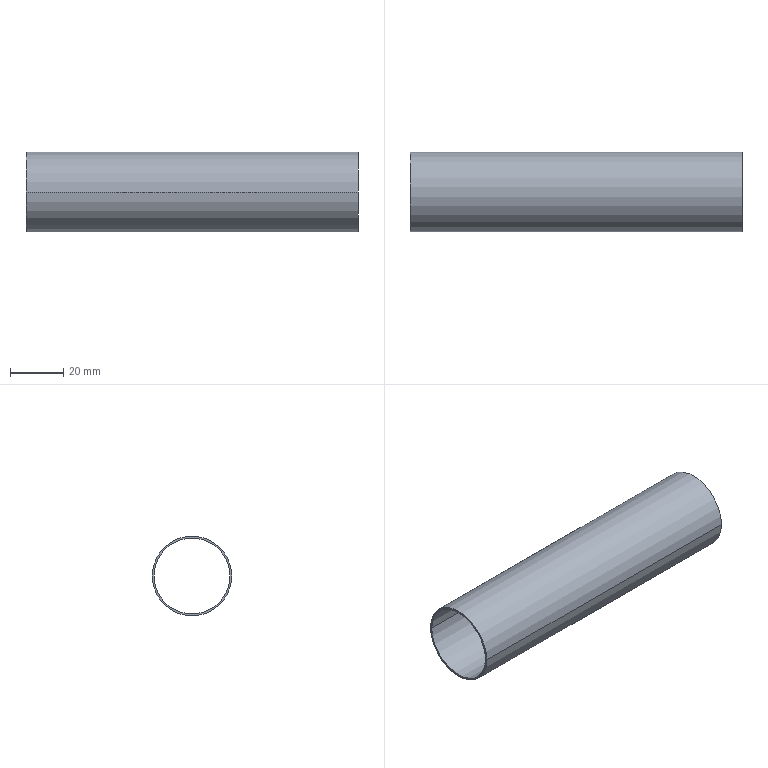Part | STEP file | Component4_2 | 1 solid | 6 faces | box 125 x 30 x 30 mm | volume 8054 mm3 | cylinder 4 | plane 2 | commonest cylinder face diameters 28.6 x2 30 x2
STEP:
#1=CARTESIAN_POINT('',(140.,140.7,17.));
#2=VERTEX_POINT('',#1);
#3=CARTESIAN_POINT('',(140.,169.3,17.));
#4=VERTEX_POINT('',#3);
#5=CARTESIAN_POINT('',(140.,155.,17.));
#6=DIRECTION('',(-1.,0.,0.));
#7=DIRECTION('',(0.,1.,0.));
#8=AXIS2_PLACEMENT_3D('',#5,#6,#7);
#9=CIRCLE('',#8,14.3);
#10=EDGE_CURVE('',#2,#4,#9,.T.);
#11=ORIENTED_EDGE('',*,*,#10,.F.);
#12=CARTESIAN_POINT('',(15.,140.7,17.));
#13=VERTEX_POINT('',#12);
#14=CARTESIAN_POINT('',(140.,140.7,17.));
#15=DIRECTION('',(-1.,0.,0.));
#16=VECTOR('',#15,1000.);
#17=LINE('',#14,#16);
#18=EDGE_CURVE('',#2,#13,#17,.T.);
#19=ORIENTED_EDGE('',*,*,#18,.T.);
#20=CARTESIAN_POINT('',(15.,169.3,17.));
#21=VERTEX_POINT('',#20);
#22=CARTESIAN_POINT('',(15.,155.,17.));
#23=DIRECTION('',(1.,0.,0.));
#24=DIRECTION('',(0.,1.,0.));
#25=AXIS2_PLACEMENT_3D('',#22,#23,#24);
#26=CIRCLE('',#25,14.3);
#27=EDGE_CURVE('',#21,#13,#26,.T.);
#28=ORIENTED_EDGE('',*,*,#27,.F.);
#29=CARTESIAN_POINT('',(140.,169.3,17.));
#30=DIRECTION('',(-1.,0.,0.));
#31=VECTOR('',#30,1000.);
#32=LINE('',#29,#31);
#33=EDGE_CURVE('',#4,#21,#32,.T.);
#34=ORIENTED_EDGE('',*,*,#33,.F.);
#35=EDGE_LOOP('',(#11,#19,#28,#34));
#36=FACE_OUTER_BOUND('',#35,.T.);
#37=CARTESIAN_POINT('',(140.,155.,17.));
#38=DIRECTION('',(-1.,0.,0.));
#39=DIRECTION('',(0.,1.,0.));
#40=AXIS2_PLACEMENT_3D('',#37,#38,#39);
#41=CYLINDRICAL_SURFACE('',#40,14.3);
#42=ADVANCED_FACE('',(#36),#41,.F.);
#43=CARTESIAN_POINT('',(140.,140.,17.));
#44=VERTEX_POINT('',#43);
#45=CARTESIAN_POINT('',(140.,170.,17.));
#46=VERTEX_POINT('',#45);
#47=CARTESIAN_POINT('',(140.,155.,17.));
#48=DIRECTION('',(1.,0.,0.));
#49=DIRECTION('',(0.,1.,0.));
#50=AXIS2_PLACEMENT_3D('',#47,#48,#49);
#51=CIRCLE('',#50,15.);
#52=EDGE_CURVE('',#44,#46,#51,.T.);
#53=ORIENTED_EDGE('',*,*,#52,.F.);
#54=CARTESIAN_POINT('',(15.,140.,17.));
#55=VERTEX_POINT('',#54);
#56=CARTESIAN_POINT('',(140.,140.,17.));
#57=DIRECTION('',(-1.,0.,0.));
#58=VECTOR('',#57,1000.);
#59=LINE('',#56,#58);
#60=EDGE_CURVE('',#44,#55,#59,.T.);
#61=ORIENTED_EDGE('',*,*,#60,.T.);
#62=CARTESIAN_POINT('',(15.,170.,17.));
#63=VERTEX_POINT('',#62);
#64=CARTESIAN_POINT('',(15.,155.,17.));
#65=DIRECTION('',(-1.,0.,0.));
#66=DIRECTION('',(0.,1.,0.));
#67=AXIS2_PLACEMENT_3D('',#64,#65,#66);
#68=CIRCLE('',#67,15.);
#69=EDGE_CURVE('',#63,#55,#68,.T.);
#70=ORIENTED_EDGE('',*,*,#69,.F.);
#71=CARTESIAN_POINT('',(140.,170.,17.));
#72=DIRECTION('',(-1.,0.,0.));
#73=VECTOR('',#72,1000.);
#74=LINE('',#71,#73);
#75=EDGE_CURVE('',#46,#63,#74,.T.);
#76=ORIENTED_EDGE('',*,*,#75,.F.);
#77=EDGE_LOOP('',(#53,#61,#70,#76));
#78=FACE_OUTER_BOUND('',#77,.T.);
#79=CARTESIAN_POINT('',(140.,155.,17.));
#80=DIRECTION('',(-1.,0.,0.));
#81=DIRECTION('',(0.,1.,0.));
#82=AXIS2_PLACEMENT_3D('',#79,#80,#81);
#83=CYLINDRICAL_SURFACE('',#82,15.);
#84=ADVANCED_FACE('',(#78),#83,.T.);
#85=ORIENTED_EDGE('',*,*,#27,.T.);
#86=CARTESIAN_POINT('',(15.,155.,17.));
#87=DIRECTION('',(1.,0.,0.));
#88=DIRECTION('',(0.,1.,0.));
#89=AXIS2_PLACEMENT_3D('',#86,#87,#88);
#90=CIRCLE('',#89,14.3);
#91=EDGE_CURVE('',#13,#21,#90,.T.);
#92=ORIENTED_EDGE('',*,*,#91,.T.);
#93=EDGE_LOOP('',(#85,#92));
#94=FACE_BOUND('',#93,.T.);
#95=ORIENTED_EDGE('',*,*,#69,.T.);
#96=CARTESIAN_POINT('',(15.,155.,17.));
#97=DIRECTION('',(-1.,0.,0.));
#98=DIRECTION('',(0.,1.,0.));
#99=AXIS2_PLACEMENT_3D('',#96,#97,#98);
#100=CIRCLE('',#99,15.);
#101=EDGE_CURVE('',#55,#63,#100,.T.);
#102=ORIENTED_EDGE('',*,*,#101,.T.);
#103=EDGE_LOOP('',(#95,#102));
#104=FACE_OUTER_BOUND('',#103,.T.);
#105=CARTESIAN_POINT('',(15.,155.,17.));
#106=DIRECTION('',(1.,0.,0.));
#107=DIRECTION('',(0.,1.,0.));
#108=AXIS2_PLACEMENT_3D('',#105,#106,#107);
#109=PLANE('',#108);
#110=ADVANCED_FACE('',(#94,#104),#109,.F.);
#111=CARTESIAN_POINT('',(140.,155.,17.));
#112=DIRECTION('',(-1.,0.,0.));
#113=DIRECTION('',(0.,1.,0.));
#114=AXIS2_PLACEMENT_3D('',#111,#112,#113);
#115=CIRCLE('',#114,14.3);
#116=EDGE_CURVE('',#4,#2,#115,.T.);
#117=ORIENTED_EDGE('',*,*,#116,.T.);
#118=ORIENTED_EDGE('',*,*,#10,.T.);
#119=EDGE_LOOP('',(#117,#118));
#120=FACE_BOUND('',#119,.T.);
#121=CARTESIAN_POINT('',(140.,155.,17.));
#122=DIRECTION('',(1.,0.,0.));
#123=DIRECTION('',(0.,1.,0.));
#124=AXIS2_PLACEMENT_3D('',#121,#122,#123);
#125=CIRCLE('',#124,15.);
#126=EDGE_CURVE('',#46,#44,#125,.T.);
#127=ORIENTED_EDGE('',*,*,#126,.T.);
#128=ORIENTED_EDGE('',*,*,#52,.T.);
#129=EDGE_LOOP('',(#127,#128));
#130=FACE_OUTER_BOUND('',#129,.T.);
#131=CARTESIAN_POINT('',(140.,155.,17.));
#132=DIRECTION('',(1.,0.,0.));
#133=DIRECTION('',(0.,1.,0.));
#134=AXIS2_PLACEMENT_3D('',#131,#132,#133);
#135=PLANE('',#134);
#136=ADVANCED_FACE('',(#120,#130),#135,.T.);
#137=ORIENTED_EDGE('',*,*,#60,.F.);
#138=ORIENTED_EDGE('',*,*,#126,.F.);
#139=ORIENTED_EDGE('',*,*,#75,.T.);
#140=ORIENTED_EDGE('',*,*,#101,.F.);
#141=EDGE_LOOP('',(#137,#138,#139,#140));
#142=FACE_OUTER_BOUND('',#141,.T.);
#143=CARTESIAN_POINT('',(140.,155.,17.));
#144=DIRECTION('',(-1.,0.,0.));
#145=DIRECTION('',(0.,1.,0.));
#146=AXIS2_PLACEMENT_3D('',#143,#144,#145);
#147=CYLINDRICAL_SURFACE('',#146,15.);
#148=ADVANCED_FACE('',(#142),#147,.T.);
#149=ORIENTED_EDGE('',*,*,#18,.F.);
#150=ORIENTED_EDGE('',*,*,#116,.F.);
#151=ORIENTED_EDGE('',*,*,#33,.T.);
#152=ORIENTED_EDGE('',*,*,#91,.F.);
#153=EDGE_LOOP('',(#149,#150,#151,#152));
#154=FACE_OUTER_BOUND('',#153,.T.);
#155=CARTESIAN_POINT('',(140.,155.,17.));
#156=DIRECTION('',(-1.,0.,0.));
#157=DIRECTION('',(0.,1.,0.));
#158=AXIS2_PLACEMENT_3D('',#155,#156,#157);
#159=CYLINDRICAL_SURFACE('',#158,14.3);
#160=ADVANCED_FACE('',(#154),#159,.F.);
#161=CLOSED_SHELL('',(#42,#84,#110,#136,#148,#160));
#162=MANIFOLD_SOLID_BREP('',#161);
#163=CARTESIAN_POINT('',(0.,0.,0.));
#164=DIRECTION('',(0.,0.,1.));
#165=DIRECTION('',(1.,0.,0.));
#166=AXIS2_PLACEMENT_3D('',#163,#164,#165);
#167=(LENGTH_UNIT()NAMED_UNIT(*)SI_UNIT(.MILLI.,.METRE.));
#168=UNCERTAINTY_MEASURE_WITH_UNIT(LENGTH_MEASURE(0.00001),#167,'','');
#169=(NAMED_UNIT(*)PLANE_ANGLE_UNIT()SI_UNIT($,.RADIAN.));
#170=(NAMED_UNIT(*)SI_UNIT($,.STERADIAN.)SOLID_ANGLE_UNIT());
#171=(GEOMETRIC_REPRESENTATION_CONTEXT(3)GLOBAL_UNCERTAINTY_ASSIGNED_CONTEXT((#168))GLOBAL_UNIT_ASSIGNED_CONTEXT((#167,#169,#170))REPRESENTATION_CONTEXT('',''));
#172=ADVANCED_BREP_SHAPE_REPRESENTATION('',(#162,#166),#171);